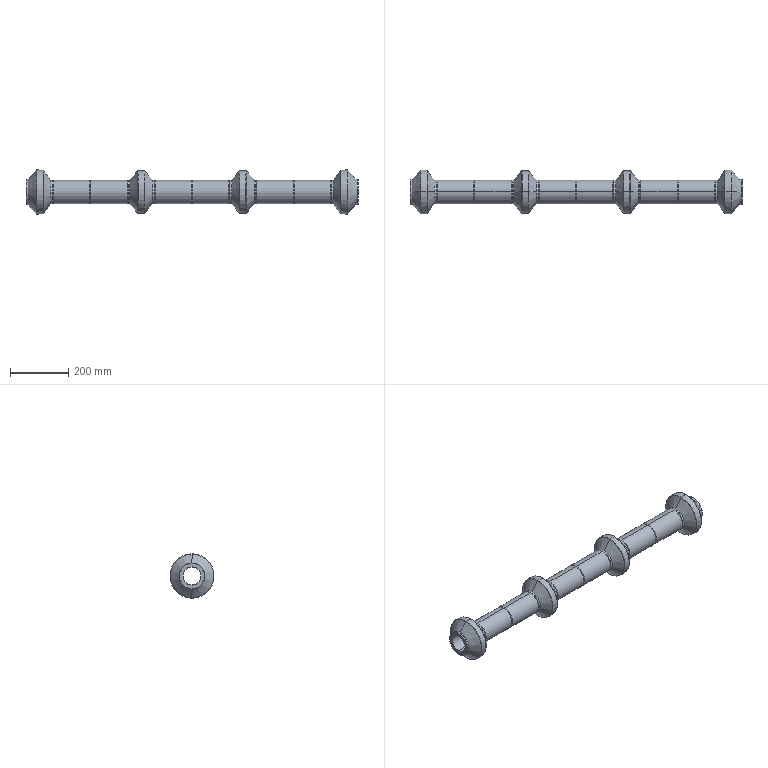Part | SolidWorks | features BaseBody 2 | 2 solids | 172 faces | box 1139 x 151.914 x 151.914 mm | volume 4895184 mm3 | cone 64 | torus 56 | cylinder 48 | plane 4 | commonest cylinder face diameters 80 x24 60 x20 146.786 x4